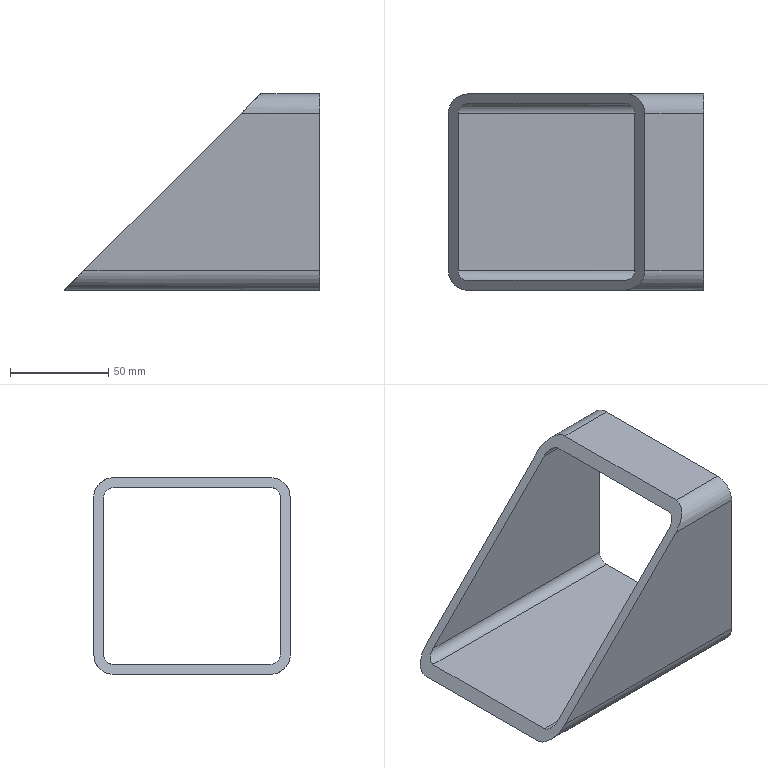Part | SolidWorks | features 3DProfileFeature 1, Cut 1, WeldMemberFeat 1, WeldmentFeature 1 | 1 solid | 18 faces | box 130 x 100 x 100 mm | volume 146850 mm3 | plane 10 | cylinder 8 | commonest cylinder face diameters 10 x4 20 x4
STEP:
#1=CARTESIAN_POINT('',(80.,50.,-40.));
#2=VERTEX_POINT('',#1);
#3=CARTESIAN_POINT('',(70.,40.,-50.));
#4=VERTEX_POINT('',#3);
#5=CARTESIAN_POINT('',(80.,50.,-40.));
#6=CARTESIAN_POINT('',(74.142,50.,-45.858));
#7=CARTESIAN_POINT('',(70.,45.858,-50.));
#8=CARTESIAN_POINT('',(70.,40.,-50.));
#9=(BOUNDED_CURVE()B_SPLINE_CURVE(3,(#5,#6,#7,#8),.UNSPECIFIED.,.F.,.F.)B_SPLINE_CURVE_WITH_KNOTS((4,4),(4.712,6.283),.UNSPECIFIED.)CURVE()GEOMETRIC_REPRESENTATION_ITEM()RATIONAL_B_SPLINE_CURVE((1.,0.8047,0.8047,1.))REPRESENTATION_ITEM(''));
#10=EDGE_CURVE('',#2,#4,#9,.T.);
#11=ORIENTED_EDGE('',*,*,#10,.F.);
#12=CARTESIAN_POINT('',(200.,50.,-40.));
#13=VERTEX_POINT('',#12);
#14=CARTESIAN_POINT('',(200.,50.,-40.));
#15=DIRECTION('',(-1.,0.,0.));
#16=VECTOR('',#15,1000.);
#17=LINE('',#14,#16);
#18=EDGE_CURVE('',#13,#2,#17,.T.);
#19=ORIENTED_EDGE('',*,*,#18,.F.);
#20=CARTESIAN_POINT('',(200.,40.,-50.));
#21=VERTEX_POINT('',#20);
#22=CARTESIAN_POINT('',(200.,40.,-40.));
#23=DIRECTION('',(1.,0.,0.));
#24=DIRECTION('',(0.,0.,-1.));
#25=AXIS2_PLACEMENT_3D('',#22,#23,#24);
#26=CIRCLE('',#25,10.);
#27=EDGE_CURVE('',#21,#13,#26,.T.);
#28=ORIENTED_EDGE('',*,*,#27,.F.);
#29=CARTESIAN_POINT('',(200.,40.,-50.));
#30=DIRECTION('',(-1.,0.,0.));
#31=VECTOR('',#30,1000.);
#32=LINE('',#29,#31);
#33=EDGE_CURVE('',#21,#4,#32,.T.);
#34=ORIENTED_EDGE('',*,*,#33,.T.);
#35=EDGE_LOOP('',(#11,#19,#28,#34));
#36=FACE_OUTER_BOUND('',#35,.T.);
#37=CARTESIAN_POINT('',(200.,40.,-40.));
#38=DIRECTION('',(-1.,0.,0.));
#39=DIRECTION('',(0.,0.,1.));
#40=AXIS2_PLACEMENT_3D('',#37,#38,#39);
#41=CYLINDRICAL_SURFACE('',#40,10.);
#42=ADVANCED_FACE('',(#36),#41,.T.);
#43=CARTESIAN_POINT('',(160.,50.,40.));
#44=VERTEX_POINT('',#43);
#45=CARTESIAN_POINT('',(170.,50.,50.));
#46=DIRECTION('',(0.7071,0.,0.7071));
#47=VECTOR('',#46,1000.);
#48=LINE('',#45,#47);
#49=EDGE_CURVE('',#2,#44,#48,.T.);
#50=ORIENTED_EDGE('',*,*,#49,.T.);
#51=CARTESIAN_POINT('',(200.,50.,40.));
#52=VERTEX_POINT('',#51);
#53=CARTESIAN_POINT('',(200.,50.,40.));
#54=DIRECTION('',(-1.,0.,0.));
#55=VECTOR('',#54,1000.);
#56=LINE('',#53,#55);
#57=EDGE_CURVE('',#52,#44,#56,.T.);
#58=ORIENTED_EDGE('',*,*,#57,.F.);
#59=CARTESIAN_POINT('',(200.,50.,-40.));
#60=DIRECTION('',(0.,0.,1.));
#61=VECTOR('',#60,1000.);
#62=LINE('',#59,#61);
#63=EDGE_CURVE('',#13,#52,#62,.T.);
#64=ORIENTED_EDGE('',*,*,#63,.F.);
#65=ORIENTED_EDGE('',*,*,#18,.T.);
#66=EDGE_LOOP('',(#50,#58,#64,#65));
#67=FACE_OUTER_BOUND('',#66,.T.);
#68=CARTESIAN_POINT('',(200.,50.,-40.));
#69=DIRECTION('',(0.,-1.,0.));
#70=DIRECTION('',(0.,0.,-1.));
#71=AXIS2_PLACEMENT_3D('',#68,#69,#70);
#72=PLANE('',#71);
#73=ADVANCED_FACE('',(#67),#72,.F.);
#74=CARTESIAN_POINT('',(170.,40.,50.));
#75=VERTEX_POINT('',#74);
#76=CARTESIAN_POINT('',(170.,40.,50.));
#77=CARTESIAN_POINT('',(170.,45.858,50.));
#78=CARTESIAN_POINT('',(165.858,50.,45.858));
#79=CARTESIAN_POINT('',(160.,50.,40.));
#80=(BOUNDED_CURVE()B_SPLINE_CURVE(3,(#76,#77,#78,#79),.UNSPECIFIED.,.F.,.F.)B_SPLINE_CURVE_WITH_KNOTS((4,4),(3.142,4.712),.UNSPECIFIED.)CURVE()GEOMETRIC_REPRESENTATION_ITEM()RATIONAL_B_SPLINE_CURVE((1.,0.8047,0.8047,1.))REPRESENTATION_ITEM(''));
#81=EDGE_CURVE('',#75,#44,#80,.T.);
#82=ORIENTED_EDGE('',*,*,#81,.F.);
#83=CARTESIAN_POINT('',(200.,40.,50.));
#84=VERTEX_POINT('',#83);
#85=CARTESIAN_POINT('',(200.,40.,50.));
#86=DIRECTION('',(-1.,0.,0.));
#87=VECTOR('',#86,1000.);
#88=LINE('',#85,#87);
#89=EDGE_CURVE('',#84,#75,#88,.T.);
#90=ORIENTED_EDGE('',*,*,#89,.F.);
#91=CARTESIAN_POINT('',(200.,40.,40.));
#92=DIRECTION('',(1.,0.,0.));
#93=DIRECTION('',(0.,0.,-1.));
#94=AXIS2_PLACEMENT_3D('',#91,#92,#93);
#95=CIRCLE('',#94,10.);
#96=EDGE_CURVE('',#52,#84,#95,.T.);
#97=ORIENTED_EDGE('',*,*,#96,.F.);
#98=ORIENTED_EDGE('',*,*,#57,.T.);
#99=EDGE_LOOP('',(#82,#90,#97,#98));
#100=FACE_OUTER_BOUND('',#99,.T.);
#101=CARTESIAN_POINT('',(200.,40.,40.));
#102=DIRECTION('',(-1.,0.,0.));
#103=DIRECTION('',(0.,0.,1.));
#104=AXIS2_PLACEMENT_3D('',#101,#102,#103);
#105=CYLINDRICAL_SURFACE('',#104,10.);
#106=ADVANCED_FACE('',(#100),#105,.T.);
#107=CARTESIAN_POINT('',(170.,-40.,50.));
#108=VERTEX_POINT('',#107);
#109=CARTESIAN_POINT('',(170.,-247.231,50.));
#110=DIRECTION('',(0.,1.,0.));
#111=VECTOR('',#110,1000.);
#112=LINE('',#109,#111);
#113=EDGE_CURVE('',#108,#75,#112,.T.);
#114=ORIENTED_EDGE('',*,*,#113,.F.);
#115=CARTESIAN_POINT('',(200.,-40.,50.));
#116=VERTEX_POINT('',#115);
#117=CARTESIAN_POINT('',(200.,-40.,50.));
#118=DIRECTION('',(-1.,0.,0.));
#119=VECTOR('',#118,1000.);
#120=LINE('',#117,#119);
#121=EDGE_CURVE('',#116,#108,#120,.T.);
#122=ORIENTED_EDGE('',*,*,#121,.F.);
#123=CARTESIAN_POINT('',(200.,-40.,50.));
#124=DIRECTION('',(0.,-1.,0.));
#125=VECTOR('',#124,1000.);
#126=LINE('',#123,#125);
#127=EDGE_CURVE('',#84,#116,#126,.T.);
#128=ORIENTED_EDGE('',*,*,#127,.F.);
#129=ORIENTED_EDGE('',*,*,#89,.T.);
#130=EDGE_LOOP('',(#114,#122,#128,#129));
#131=FACE_OUTER_BOUND('',#130,.T.);
#132=CARTESIAN_POINT('',(200.,-40.,50.));
#133=DIRECTION('',(0.,0.,-1.));
#134=DIRECTION('',(-1.,0.,0.));
#135=AXIS2_PLACEMENT_3D('',#132,#133,#134);
#136=PLANE('',#135);
#137=ADVANCED_FACE('',(#131),#136,.F.);
#138=CARTESIAN_POINT('',(160.,-50.,40.));
#139=VERTEX_POINT('',#138);
#140=CARTESIAN_POINT('',(160.,-50.,40.));
#141=CARTESIAN_POINT('',(165.858,-50.,45.858));
#142=CARTESIAN_POINT('',(170.,-45.858,50.));
#143=CARTESIAN_POINT('',(170.,-40.,50.));
#144=(BOUNDED_CURVE()B_SPLINE_CURVE(3,(#140,#141,#142,#143),.UNSPECIFIED.,.F.,.F.)B_SPLINE_CURVE_WITH_KNOTS((4,4),(1.571,3.142),.UNSPECIFIED.)CURVE()GEOMETRIC_REPRESENTATION_ITEM()RATIONAL_B_SPLINE_CURVE((1.,0.8047,0.8047,1.))REPRESENTATION_ITEM(''));
#145=EDGE_CURVE('',#139,#108,#144,.T.);
#146=ORIENTED_EDGE('',*,*,#145,.F.);
#147=CARTESIAN_POINT('',(200.,-50.,40.));
#148=VERTEX_POINT('',#147);
#149=CARTESIAN_POINT('',(200.,-50.,40.));
#150=DIRECTION('',(-1.,0.,0.));
#151=VECTOR('',#150,1000.);
#152=LINE('',#149,#151);
#153=EDGE_CURVE('',#148,#139,#152,.T.);
#154=ORIENTED_EDGE('',*,*,#153,.F.);
#155=CARTESIAN_POINT('',(200.,-40.,40.));
#156=DIRECTION('',(1.,0.,0.));
#157=DIRECTION('',(0.,0.,-1.));
#158=AXIS2_PLACEMENT_3D('',#155,#156,#157);
#159=CIRCLE('',#158,10.);
#160=EDGE_CURVE('',#116,#148,#159,.T.);
#161=ORIENTED_EDGE('',*,*,#160,.F.);
#162=ORIENTED_EDGE('',*,*,#121,.T.);
#163=EDGE_LOOP('',(#146,#154,#161,#162));
#164=FACE_OUTER_BOUND('',#163,.T.);
#165=CARTESIAN_POINT('',(200.,-40.,40.));
#166=DIRECTION('',(-1.,0.,0.));
#167=DIRECTION('',(0.,0.,1.));
#168=AXIS2_PLACEMENT_3D('',#165,#166,#167);
#169=CYLINDRICAL_SURFACE('',#168,10.);
#170=ADVANCED_FACE('',(#164),#169,.T.);
#171=CARTESIAN_POINT('',(80.,-50.,-40.));
#172=VERTEX_POINT('',#171);
#173=CARTESIAN_POINT('',(170.,-50.,50.));
#174=DIRECTION('',(-0.7071,0.,-0.7071));
#175=VECTOR('',#174,1000.);
#176=LINE('',#173,#175);
#177=EDGE_CURVE('',#139,#172,#176,.T.);
#178=ORIENTED_EDGE('',*,*,#177,.T.);
#179=CARTESIAN_POINT('',(200.,-50.,-40.));
#180=VERTEX_POINT('',#179);
#181=CARTESIAN_POINT('',(200.,-50.,-40.));
#182=DIRECTION('',(-1.,0.,0.));
#183=VECTOR('',#182,1000.);
#184=LINE('',#181,#183);
#185=EDGE_CURVE('',#180,#172,#184,.T.);
#186=ORIENTED_EDGE('',*,*,#185,.F.);
#187=CARTESIAN_POINT('',(200.,-50.,40.));
#188=DIRECTION('',(0.,0.,-1.));
#189=VECTOR('',#188,1000.);
#190=LINE('',#187,#189);
#191=EDGE_CURVE('',#148,#180,#190,.T.);
#192=ORIENTED_EDGE('',*,*,#191,.F.);
#193=ORIENTED_EDGE('',*,*,#153,.T.);
#194=EDGE_LOOP('',(#178,#186,#192,#193));
#195=FACE_OUTER_BOUND('',#194,.T.);
#196=CARTESIAN_POINT('',(200.,-50.,40.));
#197=DIRECTION('',(0.,1.,0.));
#198=DIRECTION('',(0.,0.,1.));
#199=AXIS2_PLACEMENT_3D('',#196,#197,#198);
#200=PLANE('',#199);
#201=ADVANCED_FACE('',(#195),#200,.F.);
#202=CARTESIAN_POINT('',(70.,-40.,-50.));
#203=VERTEX_POINT('',#202);
#204=CARTESIAN_POINT('',(70.,-40.,-50.));
#205=CARTESIAN_POINT('',(70.,-45.858,-50.));
#206=CARTESIAN_POINT('',(74.142,-50.,-45.858));
#207=CARTESIAN_POINT('',(80.,-50.,-40.));
#208=(BOUNDED_CURVE()B_SPLINE_CURVE(3,(#204,#205,#206,#207),.UNSPECIFIED.,.F.,.F.)B_SPLINE_CURVE_WITH_KNOTS((4,4),(0.,1.571),.UNSPECIFIED.)CURVE()GEOMETRIC_REPRESENTATION_ITEM()RATIONAL_B_SPLINE_CURVE((1.,0.8047,0.8047,1.))REPRESENTATION_ITEM(''));
#209=EDGE_CURVE('',#203,#172,#208,.T.);
#210=ORIENTED_EDGE('',*,*,#209,.F.);
#211=CARTESIAN_POINT('',(200.,-40.,-50.));
#212=VERTEX_POINT('',#211);
#213=CARTESIAN_POINT('',(200.,-40.,-50.));
#214=DIRECTION('',(-1.,0.,0.));
#215=VECTOR('',#214,1000.);
#216=LINE('',#213,#215);
#217=EDGE_CURVE('',#212,#203,#216,.T.);
#218=ORIENTED_EDGE('',*,*,#217,.F.);
#219=CARTESIAN_POINT('',(200.,-40.,-40.));
#220=DIRECTION('',(1.,0.,0.));
#221=DIRECTION('',(0.,0.,-1.));
#222=AXIS2_PLACEMENT_3D('',#219,#220,#221);
#223=CIRCLE('',#222,10.);
#224=EDGE_CURVE('',#180,#212,#223,.T.);
#225=ORIENTED_EDGE('',*,*,#224,.F.);
#226=ORIENTED_EDGE('',*,*,#185,.T.);
#227=EDGE_LOOP('',(#210,#218,#225,#226));
#228=FACE_OUTER_BOUND('',#227,.T.);
#229=CARTESIAN_POINT('',(200.,-40.,-40.));
#230=DIRECTION('',(-1.,0.,0.));
#231=DIRECTION('',(0.,0.,1.));
#232=AXIS2_PLACEMENT_3D('',#229,#230,#231);
#233=CYLINDRICAL_SURFACE('',#232,10.);
#234=ADVANCED_FACE('',(#228),#233,.T.);
#235=CARTESIAN_POINT('',(200.,40.,45.));
#236=VERTEX_POINT('',#235);
#237=CARTESIAN_POINT('',(165.,40.,45.));
#238=VERTEX_POINT('',#237);
#239=CARTESIAN_POINT('',(200.,40.,45.));
#240=DIRECTION('',(-1.,0.,0.));
#241=VECTOR('',#240,1000.);
#242=LINE('',#239,#241);
#243=EDGE_CURVE('',#236,#238,#242,.T.);
#244=ORIENTED_EDGE('',*,*,#243,.T.);
#245=CARTESIAN_POINT('',(160.,45.,40.));
#246=VERTEX_POINT('',#245);
#247=CARTESIAN_POINT('',(165.,40.,45.));
#248=CARTESIAN_POINT('',(165.,42.929,45.));
#249=CARTESIAN_POINT('',(162.929,45.,42.929));
#250=CARTESIAN_POINT('',(160.,45.,40.));
#251=(BOUNDED_CURVE()B_SPLINE_CURVE(3,(#247,#248,#249,#250),.UNSPECIFIED.,.F.,.F.)B_SPLINE_CURVE_WITH_KNOTS((4,4),(3.142,4.712),.UNSPECIFIED.)CURVE()GEOMETRIC_REPRESENTATION_ITEM()RATIONAL_B_SPLINE_CURVE((1.,0.8047,0.8047,1.))REPRESENTATION_ITEM(''));
#252=EDGE_CURVE('',#238,#246,#251,.T.);
#253=ORIENTED_EDGE('',*,*,#252,.T.);
#254=CARTESIAN_POINT('',(200.,45.,40.));
#255=VERTEX_POINT('',#254);
#256=CARTESIAN_POINT('',(200.,45.,40.));
#257=DIRECTION('',(-1.,0.,0.));
#258=VECTOR('',#257,1000.);
#259=LINE('',#256,#258);
#260=EDGE_CURVE('',#255,#246,#259,.T.);
#261=ORIENTED_EDGE('',*,*,#260,.F.);
#262=CARTESIAN_POINT('',(200.,40.,40.));
#263=DIRECTION('',(1.,0.,0.));
#264=DIRECTION('',(0.,0.,-1.));
#265=AXIS2_PLACEMENT_3D('',#262,#263,#264);
#266=CIRCLE('',#265,5.);
#267=EDGE_CURVE('',#255,#236,#266,.T.);
#268=ORIENTED_EDGE('',*,*,#267,.T.);
#269=EDGE_LOOP('',(#244,#253,#261,#268));
#270=FACE_OUTER_BOUND('',#269,.T.);
#271=CARTESIAN_POINT('',(200.,40.,40.));
#272=DIRECTION('',(-1.,0.,0.));
#273=DIRECTION('',(0.,0.,1.));
#274=AXIS2_PLACEMENT_3D('',#271,#272,#273);
#275=CYLINDRICAL_SURFACE('',#274,5.);
#276=ADVANCED_FACE('',(#270),#275,.F.);
#277=ORIENTED_EDGE('',*,*,#260,.T.);
#278=CARTESIAN_POINT('',(80.,45.,-40.));
#279=VERTEX_POINT('',#278);
#280=CARTESIAN_POINT('',(140.,45.,20.));
#281=DIRECTION('',(-0.7071,0.,-0.7071));
#282=VECTOR('',#281,1000.);
#283=LINE('',#280,#282);
#284=EDGE_CURVE('',#246,#279,#283,.T.);
#285=ORIENTED_EDGE('',*,*,#284,.T.);
#286=CARTESIAN_POINT('',(200.,45.,-40.));
#287=VERTEX_POINT('',#286);
#288=CARTESIAN_POINT('',(200.,45.,-40.));
#289=DIRECTION('',(-1.,0.,0.));
#290=VECTOR('',#289,1000.);
#291=LINE('',#288,#290);
#292=EDGE_CURVE('',#287,#279,#291,.T.);
#293=ORIENTED_EDGE('',*,*,#292,.F.);
#294=CARTESIAN_POINT('',(200.,45.,-40.));
#295=DIRECTION('',(0.,0.,1.));
#296=VECTOR('',#295,1000.);
#297=LINE('',#294,#296);
#298=EDGE_CURVE('',#287,#255,#297,.T.);
#299=ORIENTED_EDGE('',*,*,#298,.T.);
#300=EDGE_LOOP('',(#277,#285,#293,#299));
#301=FACE_OUTER_BOUND('',#300,.T.);
#302=CARTESIAN_POINT('',(200.,45.,-40.));
#303=DIRECTION('',(0.,-1.,0.));
#304=DIRECTION('',(0.,0.,-1.));
#305=AXIS2_PLACEMENT_3D('',#302,#303,#304);
#306=PLANE('',#305);
#307=ADVANCED_FACE('',(#301),#306,.T.);
#308=ORIENTED_EDGE('',*,*,#292,.T.);
#309=CARTESIAN_POINT('',(75.,40.,-45.));
#310=VERTEX_POINT('',#309);
#311=CARTESIAN_POINT('',(80.,45.,-40.));
#312=CARTESIAN_POINT('',(77.071,45.,-42.929));
#313=CARTESIAN_POINT('',(75.,42.929,-45.));
#314=CARTESIAN_POINT('',(75.,40.,-45.));
#315=(BOUNDED_CURVE()B_SPLINE_CURVE(3,(#311,#312,#313,#314),.UNSPECIFIED.,.F.,.F.)B_SPLINE_CURVE_WITH_KNOTS((4,4),(4.712,6.283),.UNSPECIFIED.)CURVE()GEOMETRIC_REPRESENTATION_ITEM()RATIONAL_B_SPLINE_CURVE((1.,0.8047,0.8047,1.))REPRESENTATION_ITEM(''));
#316=EDGE_CURVE('',#279,#310,#315,.T.);
#317=ORIENTED_EDGE('',*,*,#316,.T.);
#318=CARTESIAN_POINT('',(200.,40.,-45.));
#319=VERTEX_POINT('',#318);
#320=CARTESIAN_POINT('',(200.,40.,-45.));
#321=DIRECTION('',(-1.,0.,0.));
#322=VECTOR('',#321,1000.);
#323=LINE('',#320,#322);
#324=EDGE_CURVE('',#319,#310,#323,.T.);
#325=ORIENTED_EDGE('',*,*,#324,.F.);
#326=CARTESIAN_POINT('',(200.,40.,-40.));
#327=DIRECTION('',(1.,0.,0.));
#328=DIRECTION('',(0.,0.,-1.));
#329=AXIS2_PLACEMENT_3D('',#326,#327,#328);
#330=CIRCLE('',#329,5.);
#331=EDGE_CURVE('',#319,#287,#330,.T.);
#332=ORIENTED_EDGE('',*,*,#331,.T.);
#333=EDGE_LOOP('',(#308,#317,#325,#332));
#334=FACE_OUTER_BOUND('',#333,.T.);
#335=CARTESIAN_POINT('',(200.,40.,-40.));
#336=DIRECTION('',(-1.,0.,0.));
#337=DIRECTION('',(0.,0.,1.));
#338=AXIS2_PLACEMENT_3D('',#335,#336,#337);
#339=CYLINDRICAL_SURFACE('',#338,5.);
#340=ADVANCED_FACE('',(#334),#339,.F.);
#341=ORIENTED_EDGE('',*,*,#324,.T.);
#342=CARTESIAN_POINT('',(75.,-40.,-45.));
#343=VERTEX_POINT('',#342);
#344=CARTESIAN_POINT('',(75.,40.,-45.));
#345=DIRECTION('',(0.,-1.,0.));
#346=VECTOR('',#345,1000.);
#347=LINE('',#344,#346);
#348=EDGE_CURVE('',#310,#343,#347,.T.);
#349=ORIENTED_EDGE('',*,*,#348,.T.);
#350=CARTESIAN_POINT('',(200.,-40.,-45.));
#351=VERTEX_POINT('',#350);
#352=CARTESIAN_POINT('',(200.,-40.,-45.));
#353=DIRECTION('',(-1.,0.,0.));
#354=VECTOR('',#353,1000.);
#355=LINE('',#352,#354);
#356=EDGE_CURVE('',#351,#343,#355,.T.);
#357=ORIENTED_EDGE('',*,*,#356,.F.);
#358=CARTESIAN_POINT('',(200.,40.,-45.));
#359=DIRECTION('',(0.,1.,0.));
#360=VECTOR('',#359,1000.);
#361=LINE('',#358,#360);
#362=EDGE_CURVE('',#351,#319,#361,.T.);
#363=ORIENTED_EDGE('',*,*,#362,.T.);
#364=EDGE_LOOP('',(#341,#349,#357,#363));
#365=FACE_OUTER_BOUND('',#364,.T.);
#366=CARTESIAN_POINT('',(200.,40.,-45.));
#367=DIRECTION('',(0.,0.,1.));
#368=DIRECTION('',(1.,0.,0.));
#369=AXIS2_PLACEMENT_3D('',#366,#367,#368);
#370=PLANE('',#369);
#371=ADVANCED_FACE('',(#365),#370,.T.);
#372=ORIENTED_EDGE('',*,*,#356,.T.);
#373=CARTESIAN_POINT('',(80.,-45.,-40.));
#374=VERTEX_POINT('',#373);
#375=CARTESIAN_POINT('',(75.,-40.,-45.));
#376=CARTESIAN_POINT('',(75.,-42.929,-45.));
#377=CARTESIAN_POINT('',(77.071,-45.,-42.929));
#378=CARTESIAN_POINT('',(80.,-45.,-40.));
#379=(BOUNDED_CURVE()B_SPLINE_CURVE(3,(#375,#376,#377,#378),.UNSPECIFIED.,.F.,.F.)B_SPLINE_CURVE_WITH_KNOTS((4,4),(0.,1.571),.UNSPECIFIED.)CURVE()GEOMETRIC_REPRESENTATION_ITEM()RATIONAL_B_SPLINE_CURVE((1.,0.8047,0.8047,1.))REPRESENTATION_ITEM(''));
#380=EDGE_CURVE('',#343,#374,#379,.T.);
#381=ORIENTED_EDGE('',*,*,#380,.T.);
#382=CARTESIAN_POINT('',(200.,-45.,-40.));
#383=VERTEX_POINT('',#382);
#384=CARTESIAN_POINT('',(200.,-45.,-40.));
#385=DIRECTION('',(-1.,0.,0.));
#386=VECTOR('',#385,1000.);
#387=LINE('',#384,#386);
#388=EDGE_CURVE('',#383,#374,#387,.T.);
#389=ORIENTED_EDGE('',*,*,#388,.F.);
#390=CARTESIAN_POINT('',(200.,-40.,-40.));
#391=DIRECTION('',(1.,0.,0.));
#392=DIRECTION('',(0.,0.,-1.));
#393=AXIS2_PLACEMENT_3D('',#390,#391,#392);
#394=CIRCLE('',#393,5.);
#395=EDGE_CURVE('',#383,#351,#394,.T.);
#396=ORIENTED_EDGE('',*,*,#395,.T.);
#397=EDGE_LOOP('',(#372,#381,#389,#396));
#398=FACE_OUTER_BOUND('',#397,.T.);
#399=CARTESIAN_POINT('',(200.,-40.,-40.));
#400=DIRECTION('',(-1.,0.,0.));
#401=DIRECTION('',(0.,0.,1.));
#402=AXIS2_PLACEMENT_3D('',#399,#400,#401);
#403=CYLINDRICAL_SURFACE('',#402,5.);
#404=ADVANCED_FACE('',(#398),#403,.F.);
#405=ORIENTED_EDGE('',*,*,#388,.T.);
#406=CARTESIAN_POINT('',(160.,-45.,40.));
#407=VERTEX_POINT('',#406);
#408=CARTESIAN_POINT('',(180.,-45.,60.));
#409=DIRECTION('',(0.7071,0.,0.7071));
#410=VECTOR('',#409,1000.);
#411=LINE('',#408,#410);
#412=EDGE_CURVE('',#374,#407,#411,.T.);
#413=ORIENTED_EDGE('',*,*,#412,.T.);
#414=CARTESIAN_POINT('',(200.,-45.,40.));
#415=VERTEX_POINT('',#414);
#416=CARTESIAN_POINT('',(200.,-45.,40.));
#417=DIRECTION('',(-1.,0.,0.));
#418=VECTOR('',#417,1000.);
#419=LINE('',#416,#418);
#420=EDGE_CURVE('',#415,#407,#419,.T.);
#421=ORIENTED_EDGE('',*,*,#420,.F.);
#422=CARTESIAN_POINT('',(200.,-45.,40.));
#423=DIRECTION('',(0.,0.,-1.));
#424=VECTOR('',#423,1000.);
#425=LINE('',#422,#424);
#426=EDGE_CURVE('',#415,#383,#425,.T.);
#427=ORIENTED_EDGE('',*,*,#426,.T.);
#428=EDGE_LOOP('',(#405,#413,#421,#427));
#429=FACE_OUTER_BOUND('',#428,.T.);
#430=CARTESIAN_POINT('',(200.,-45.,40.));
#431=DIRECTION('',(0.,1.,0.));
#432=DIRECTION('',(0.,0.,1.));
#433=AXIS2_PLACEMENT_3D('',#430,#431,#432);
#434=PLANE('',#433);
#435=ADVANCED_FACE('',(#429),#434,.T.);
#436=ORIENTED_EDGE('',*,*,#420,.T.);
#437=CARTESIAN_POINT('',(165.,-40.,45.));
#438=VERTEX_POINT('',#437);
#439=CARTESIAN_POINT('',(160.,-45.,40.));
#440=CARTESIAN_POINT('',(162.929,-45.,42.929));
#441=CARTESIAN_POINT('',(165.,-42.929,45.));
#442=CARTESIAN_POINT('',(165.,-40.,45.));
#443=(BOUNDED_CURVE()B_SPLINE_CURVE(3,(#439,#440,#441,#442),.UNSPECIFIED.,.F.,.F.)B_SPLINE_CURVE_WITH_KNOTS((4,4),(1.571,3.142),.UNSPECIFIED.)CURVE()GEOMETRIC_REPRESENTATION_ITEM()RATIONAL_B_SPLINE_CURVE((1.,0.8047,0.8047,1.))REPRESENTATION_ITEM(''));
#444=EDGE_CURVE('',#407,#438,#443,.T.);
#445=ORIENTED_EDGE('',*,*,#444,.T.);
#446=CARTESIAN_POINT('',(200.,-40.,45.));
#447=VERTEX_POINT('',#446);
#448=CARTESIAN_POINT('',(200.,-40.,45.));
#449=DIRECTION('',(-1.,0.,0.));
#450=VECTOR('',#449,1000.);
#451=LINE('',#448,#450);
#452=EDGE_CURVE('',#447,#438,#451,.T.);
#453=ORIENTED_EDGE('',*,*,#452,.F.);
#454=CARTESIAN_POINT('',(200.,-40.,40.));
#455=DIRECTION('',(1.,0.,0.));
#456=DIRECTION('',(0.,0.,-1.));
#457=AXIS2_PLACEMENT_3D('',#454,#455,#456);
#458=CIRCLE('',#457,5.);
#459=EDGE_CURVE('',#447,#415,#458,.T.);
#460=ORIENTED_EDGE('',*,*,#459,.T.);
#461=EDGE_LOOP('',(#436,#445,#453,#460));
#462=FACE_OUTER_BOUND('',#461,.T.);
#463=CARTESIAN_POINT('',(200.,-40.,40.));
#464=DIRECTION('',(-1.,0.,0.));
#465=DIRECTION('',(0.,0.,1.));
#466=AXIS2_PLACEMENT_3D('',#463,#464,#465);
#467=CYLINDRICAL_SURFACE('',#466,5.);
#468=ADVANCED_FACE('',(#462),#467,.F.);
#469=ORIENTED_EDGE('',*,*,#452,.T.);
#470=CARTESIAN_POINT('',(165.,-40.,45.));
#471=DIRECTION('',(0.,1.,0.));
#472=VECTOR('',#471,1000.);
#473=LINE('',#470,#472);
#474=EDGE_CURVE('',#438,#238,#473,.T.);
#475=ORIENTED_EDGE('',*,*,#474,.T.);
#476=ORIENTED_EDGE('',*,*,#243,.F.);
#477=CARTESIAN_POINT('',(200.,-40.,45.));
#478=DIRECTION('',(0.,-1.,0.));
#479=VECTOR('',#478,1000.);
#480=LINE('',#477,#479);
#481=EDGE_CURVE('',#236,#447,#480,.T.);
#482=ORIENTED_EDGE('',*,*,#481,.T.);
#483=EDGE_LOOP('',(#469,#475,#476,#482));
#484=FACE_OUTER_BOUND('',#483,.T.);
#485=CARTESIAN_POINT('',(200.,-40.,45.));
#486=DIRECTION('',(0.,0.,-1.));
#487=DIRECTION('',(-1.,0.,0.));
#488=AXIS2_PLACEMENT_3D('',#485,#486,#487);
#489=PLANE('',#488);
#490=ADVANCED_FACE('',(#484),#489,.T.);
#491=CARTESIAN_POINT('',(70.,-247.231,-50.));
#492=DIRECTION('',(0.,1.,0.));
#493=VECTOR('',#492,1000.);
#494=LINE('',#491,#493);
#495=EDGE_CURVE('',#203,#4,#494,.T.);
#496=ORIENTED_EDGE('',*,*,#495,.T.);
#497=ORIENTED_EDGE('',*,*,#33,.F.);
#498=CARTESIAN_POINT('',(200.,40.,-50.));
#499=DIRECTION('',(0.,1.,0.));
#500=VECTOR('',#499,1000.);
#501=LINE('',#498,#500);
#502=EDGE_CURVE('',#212,#21,#501,.T.);
#503=ORIENTED_EDGE('',*,*,#502,.F.);
#504=ORIENTED_EDGE('',*,*,#217,.T.);
#505=EDGE_LOOP('',(#496,#497,#503,#504));
#506=FACE_OUTER_BOUND('',#505,.T.);
#507=CARTESIAN_POINT('',(200.,40.,-50.));
#508=DIRECTION('',(0.,0.,1.));
#509=DIRECTION('',(1.,0.,0.));
#510=AXIS2_PLACEMENT_3D('',#507,#508,#509);
#511=PLANE('',#510);
#512=ADVANCED_FACE('',(#506),#511,.F.);
#513=ORIENTED_EDGE('',*,*,#267,.F.);
#514=ORIENTED_EDGE('',*,*,#298,.F.);
#515=ORIENTED_EDGE('',*,*,#331,.F.);
#516=ORIENTED_EDGE('',*,*,#362,.F.);
#517=ORIENTED_EDGE('',*,*,#395,.F.);
#518=ORIENTED_EDGE('',*,*,#426,.F.);
#519=ORIENTED_EDGE('',*,*,#459,.F.);
#520=ORIENTED_EDGE('',*,*,#481,.F.);
#521=EDGE_LOOP('',(#513,#514,#515,#516,#517,#518,#519,#520));
#522=FACE_BOUND('',#521,.T.);
#523=ORIENTED_EDGE('',*,*,#27,.T.);
#524=ORIENTED_EDGE('',*,*,#63,.T.);
#525=ORIENTED_EDGE('',*,*,#96,.T.);
#526=ORIENTED_EDGE('',*,*,#127,.T.);
#527=ORIENTED_EDGE('',*,*,#160,.T.);
#528=ORIENTED_EDGE('',*,*,#191,.T.);
#529=ORIENTED_EDGE('',*,*,#224,.T.);
#530=ORIENTED_EDGE('',*,*,#502,.T.);
#531=EDGE_LOOP('',(#523,#524,#525,#526,#527,#528,#529,#530));
#532=FACE_OUTER_BOUND('',#531,.T.);
#533=CARTESIAN_POINT('',(200.,40.,-40.));
#534=DIRECTION('',(1.,0.,0.));
#535=DIRECTION('',(0.,0.,-1.));
#536=AXIS2_PLACEMENT_3D('',#533,#534,#535);
#537=PLANE('',#536);
#538=ADVANCED_FACE('',(#522,#532),#537,.T.);
#539=ORIENTED_EDGE('',*,*,#474,.F.);
#540=ORIENTED_EDGE('',*,*,#444,.F.);
#541=ORIENTED_EDGE('',*,*,#412,.F.);
#542=ORIENTED_EDGE('',*,*,#380,.F.);
#543=ORIENTED_EDGE('',*,*,#348,.F.);
#544=ORIENTED_EDGE('',*,*,#316,.F.);
#545=ORIENTED_EDGE('',*,*,#284,.F.);
#546=ORIENTED_EDGE('',*,*,#252,.F.);
#547=EDGE_LOOP('',(#539,#540,#541,#542,#543,#544,#545,#546));
#548=FACE_BOUND('',#547,.T.);
#549=ORIENTED_EDGE('',*,*,#10,.T.);
#550=ORIENTED_EDGE('',*,*,#495,.F.);
#551=ORIENTED_EDGE('',*,*,#209,.T.);
#552=ORIENTED_EDGE('',*,*,#177,.F.);
#553=ORIENTED_EDGE('',*,*,#145,.T.);
#554=ORIENTED_EDGE('',*,*,#113,.T.);
#555=ORIENTED_EDGE('',*,*,#81,.T.);
#556=ORIENTED_EDGE('',*,*,#49,.F.);
#557=EDGE_LOOP('',(#549,#550,#551,#552,#553,#554,#555,#556));
#558=FACE_OUTER_BOUND('',#557,.T.);
#559=CARTESIAN_POINT('',(170.,-247.231,50.));
#560=DIRECTION('',(-0.7071,0.,0.7071));
#561=DIRECTION('',(0.7071,0.,0.7071));
#562=AXIS2_PLACEMENT_3D('',#559,#560,#561);
#563=PLANE('',#562);
#564=ADVANCED_FACE('',(#548,#558),#563,.T.);
#565=CLOSED_SHELL('',(#42,#73,#106,#137,#170,#201,#234,#276,#307,#340,#371,#404,#435,#468,#490,#512,#538,#564));
#566=MANIFOLD_SOLID_BREP('',#565);
#567=CARTESIAN_POINT('',(0.,0.,0.));
#568=DIRECTION('',(0.,0.,1.));
#569=DIRECTION('',(1.,0.,0.));
#570=AXIS2_PLACEMENT_3D('',#567,#568,#569);
#571=(LENGTH_UNIT()NAMED_UNIT(*)SI_UNIT(.MILLI.,.METRE.));
#572=UNCERTAINTY_MEASURE_WITH_UNIT(LENGTH_MEASURE(0.00001),#571,'','');
#573=(NAMED_UNIT(*)PLANE_ANGLE_UNIT()SI_UNIT($,.RADIAN.));
#574=(NAMED_UNIT(*)SI_UNIT($,.STERADIAN.)SOLID_ANGLE_UNIT());
#575=(GEOMETRIC_REPRESENTATION_CONTEXT(3)GLOBAL_UNCERTAINTY_ASSIGNED_CONTEXT((#572))GLOBAL_UNIT_ASSIGNED_CONTEXT((#571,#573,#574))REPRESENTATION_CONTEXT('',''));
#576=ADVANCED_BREP_SHAPE_REPRESENTATION('',(#566,#570),#575);